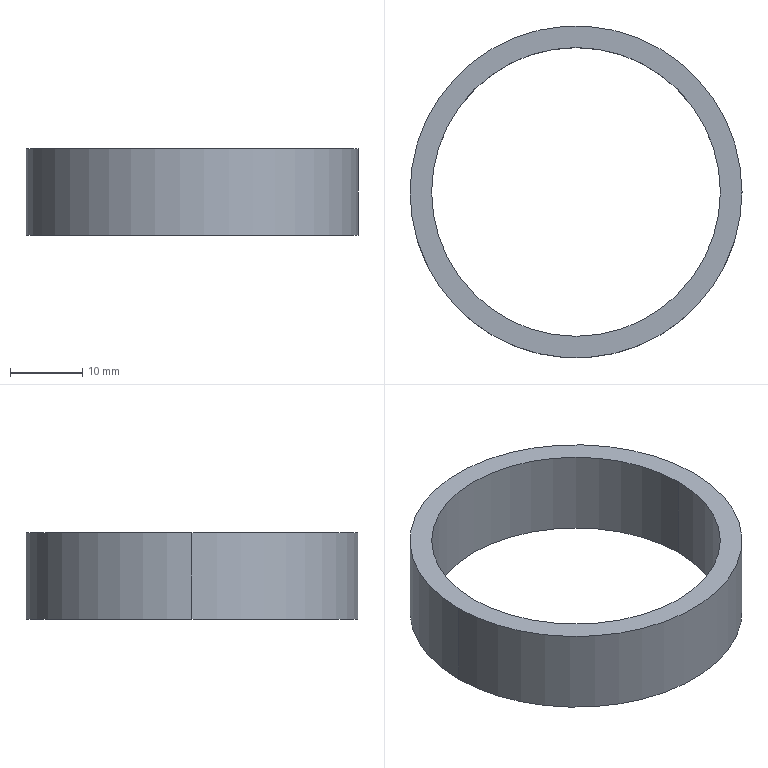Part | SolidWorks | features Extrusion 1 | 1 solid | 6 faces | box 46 x 46 x 12 mm | volume 4863 mm3 | cylinder 4 | plane 2 | commonest cylinder face diameters 40 x2 46 x2
STEP:
#1=CARTESIAN_POINT('',(-20.,0.,12.));
#2=VERTEX_POINT('',#1);
#3=CARTESIAN_POINT('',(20.,0.,12.));
#4=VERTEX_POINT('',#3);
#5=CARTESIAN_POINT('',(0.,0.,12.));
#6=DIRECTION('',(0.,0.,1.));
#7=DIRECTION('',(1.,0.,0.));
#8=AXIS2_PLACEMENT_3D('',#5,#6,#7);
#9=CIRCLE('',#8,20.);
#10=EDGE_CURVE('',#2,#4,#9,.T.);
#11=ORIENTED_EDGE('',*,*,#10,.T.);
#12=CARTESIAN_POINT('',(20.,0.,0.));
#13=VERTEX_POINT('',#12);
#14=CARTESIAN_POINT('',(20.,0.,12.));
#15=DIRECTION('',(0.,0.,-1.));
#16=VECTOR('',#15,1000.);
#17=LINE('',#14,#16);
#18=EDGE_CURVE('',#4,#13,#17,.T.);
#19=ORIENTED_EDGE('',*,*,#18,.T.);
#20=CARTESIAN_POINT('',(-20.,0.,0.));
#21=VERTEX_POINT('',#20);
#22=CARTESIAN_POINT('',(0.,0.,0.));
#23=DIRECTION('',(0.,0.,1.));
#24=DIRECTION('',(1.,0.,0.));
#25=AXIS2_PLACEMENT_3D('',#22,#23,#24);
#26=CIRCLE('',#25,20.);
#27=EDGE_CURVE('',#21,#13,#26,.T.);
#28=ORIENTED_EDGE('',*,*,#27,.F.);
#29=CARTESIAN_POINT('',(-20.,0.,12.));
#30=DIRECTION('',(0.,0.,-1.));
#31=VECTOR('',#30,1000.);
#32=LINE('',#29,#31);
#33=EDGE_CURVE('',#2,#21,#32,.T.);
#34=ORIENTED_EDGE('',*,*,#33,.F.);
#35=EDGE_LOOP('',(#11,#19,#28,#34));
#36=FACE_OUTER_BOUND('',#35,.T.);
#37=CARTESIAN_POINT('',(0.,0.,12.));
#38=DIRECTION('',(0.,0.,-1.));
#39=DIRECTION('',(-1.,0.,0.));
#40=AXIS2_PLACEMENT_3D('',#37,#38,#39);
#41=CYLINDRICAL_SURFACE('',#40,20.);
#42=ADVANCED_FACE('',(#36),#41,.F.);
#43=CARTESIAN_POINT('',(23.,0.,12.));
#44=VERTEX_POINT('',#43);
#45=CARTESIAN_POINT('',(-23.,0.,12.));
#46=VERTEX_POINT('',#45);
#47=CARTESIAN_POINT('',(0.,0.,12.));
#48=DIRECTION('',(0.,0.,1.));
#49=DIRECTION('',(1.,0.,0.));
#50=AXIS2_PLACEMENT_3D('',#47,#48,#49);
#51=CIRCLE('',#50,23.);
#52=EDGE_CURVE('',#44,#46,#51,.T.);
#53=ORIENTED_EDGE('',*,*,#52,.F.);
#54=CARTESIAN_POINT('',(23.,0.,0.));
#55=VERTEX_POINT('',#54);
#56=CARTESIAN_POINT('',(23.,0.,12.));
#57=DIRECTION('',(0.,0.,-1.));
#58=VECTOR('',#57,1000.);
#59=LINE('',#56,#58);
#60=EDGE_CURVE('',#44,#55,#59,.T.);
#61=ORIENTED_EDGE('',*,*,#60,.T.);
#62=CARTESIAN_POINT('',(-23.,0.,0.));
#63=VERTEX_POINT('',#62);
#64=CARTESIAN_POINT('',(0.,0.,0.));
#65=DIRECTION('',(0.,0.,1.));
#66=DIRECTION('',(1.,0.,0.));
#67=AXIS2_PLACEMENT_3D('',#64,#65,#66);
#68=CIRCLE('',#67,23.);
#69=EDGE_CURVE('',#55,#63,#68,.T.);
#70=ORIENTED_EDGE('',*,*,#69,.T.);
#71=CARTESIAN_POINT('',(-23.,0.,12.));
#72=DIRECTION('',(0.,0.,-1.));
#73=VECTOR('',#72,1000.);
#74=LINE('',#71,#73);
#75=EDGE_CURVE('',#46,#63,#74,.T.);
#76=ORIENTED_EDGE('',*,*,#75,.F.);
#77=EDGE_LOOP('',(#53,#61,#70,#76));
#78=FACE_OUTER_BOUND('',#77,.T.);
#79=CARTESIAN_POINT('',(0.,0.,12.));
#80=DIRECTION('',(0.,0.,-1.));
#81=DIRECTION('',(-1.,0.,0.));
#82=AXIS2_PLACEMENT_3D('',#79,#80,#81);
#83=CYLINDRICAL_SURFACE('',#82,23.);
#84=ADVANCED_FACE('',(#78),#83,.T.);
#85=CARTESIAN_POINT('',(0.,0.,12.));
#86=DIRECTION('',(0.,0.,1.));
#87=DIRECTION('',(1.,0.,0.));
#88=AXIS2_PLACEMENT_3D('',#85,#86,#87);
#89=CIRCLE('',#88,23.);
#90=EDGE_CURVE('',#46,#44,#89,.T.);
#91=ORIENTED_EDGE('',*,*,#90,.T.);
#92=ORIENTED_EDGE('',*,*,#52,.T.);
#93=EDGE_LOOP('',(#91,#92));
#94=FACE_OUTER_BOUND('',#93,.T.);
#95=ORIENTED_EDGE('',*,*,#10,.F.);
#96=CARTESIAN_POINT('',(0.,0.,12.));
#97=DIRECTION('',(0.,0.,1.));
#98=DIRECTION('',(1.,0.,0.));
#99=AXIS2_PLACEMENT_3D('',#96,#97,#98);
#100=CIRCLE('',#99,20.);
#101=EDGE_CURVE('',#4,#2,#100,.T.);
#102=ORIENTED_EDGE('',*,*,#101,.F.);
#103=EDGE_LOOP('',(#95,#102));
#104=FACE_BOUND('',#103,.T.);
#105=CARTESIAN_POINT('',(0.,0.,12.));
#106=DIRECTION('',(0.,0.,1.));
#107=DIRECTION('',(1.,0.,0.));
#108=AXIS2_PLACEMENT_3D('',#105,#106,#107);
#109=PLANE('',#108);
#110=ADVANCED_FACE('',(#94,#104),#109,.T.);
#111=CARTESIAN_POINT('',(0.,0.,0.));
#112=DIRECTION('',(0.,0.,1.));
#113=DIRECTION('',(1.,0.,0.));
#114=AXIS2_PLACEMENT_3D('',#111,#112,#113);
#115=CIRCLE('',#114,23.);
#116=EDGE_CURVE('',#63,#55,#115,.T.);
#117=ORIENTED_EDGE('',*,*,#116,.F.);
#118=ORIENTED_EDGE('',*,*,#69,.F.);
#119=EDGE_LOOP('',(#117,#118));
#120=FACE_OUTER_BOUND('',#119,.T.);
#121=ORIENTED_EDGE('',*,*,#27,.T.);
#122=CARTESIAN_POINT('',(0.,0.,0.));
#123=DIRECTION('',(0.,0.,1.));
#124=DIRECTION('',(1.,0.,0.));
#125=AXIS2_PLACEMENT_3D('',#122,#123,#124);
#126=CIRCLE('',#125,20.);
#127=EDGE_CURVE('',#13,#21,#126,.T.);
#128=ORIENTED_EDGE('',*,*,#127,.T.);
#129=EDGE_LOOP('',(#121,#128));
#130=FACE_BOUND('',#129,.T.);
#131=CARTESIAN_POINT('',(0.,0.,0.));
#132=DIRECTION('',(0.,0.,1.));
#133=DIRECTION('',(1.,0.,0.));
#134=AXIS2_PLACEMENT_3D('',#131,#132,#133);
#135=PLANE('',#134);
#136=ADVANCED_FACE('',(#120,#130),#135,.F.);
#137=ORIENTED_EDGE('',*,*,#60,.F.);
#138=ORIENTED_EDGE('',*,*,#90,.F.);
#139=ORIENTED_EDGE('',*,*,#75,.T.);
#140=ORIENTED_EDGE('',*,*,#116,.T.);
#141=EDGE_LOOP('',(#137,#138,#139,#140));
#142=FACE_OUTER_BOUND('',#141,.T.);
#143=CARTESIAN_POINT('',(0.,0.,12.));
#144=DIRECTION('',(0.,0.,-1.));
#145=DIRECTION('',(-1.,0.,0.));
#146=AXIS2_PLACEMENT_3D('',#143,#144,#145);
#147=CYLINDRICAL_SURFACE('',#146,23.);
#148=ADVANCED_FACE('',(#142),#147,.T.);
#149=ORIENTED_EDGE('',*,*,#18,.F.);
#150=ORIENTED_EDGE('',*,*,#101,.T.);
#151=ORIENTED_EDGE('',*,*,#33,.T.);
#152=ORIENTED_EDGE('',*,*,#127,.F.);
#153=EDGE_LOOP('',(#149,#150,#151,#152));
#154=FACE_OUTER_BOUND('',#153,.T.);
#155=CARTESIAN_POINT('',(0.,0.,12.));
#156=DIRECTION('',(0.,0.,-1.));
#157=DIRECTION('',(-1.,0.,0.));
#158=AXIS2_PLACEMENT_3D('',#155,#156,#157);
#159=CYLINDRICAL_SURFACE('',#158,20.);
#160=ADVANCED_FACE('',(#154),#159,.F.);
#161=CLOSED_SHELL('',(#42,#84,#110,#136,#148,#160));
#162=MANIFOLD_SOLID_BREP('',#161);
#163=CARTESIAN_POINT('',(0.,0.,0.));
#164=DIRECTION('',(0.,0.,1.));
#165=DIRECTION('',(1.,0.,0.));
#166=AXIS2_PLACEMENT_3D('',#163,#164,#165);
#167=(LENGTH_UNIT()NAMED_UNIT(*)SI_UNIT(.MILLI.,.METRE.));
#168=UNCERTAINTY_MEASURE_WITH_UNIT(LENGTH_MEASURE(0.00001),#167,'','');
#169=(NAMED_UNIT(*)PLANE_ANGLE_UNIT()SI_UNIT($,.RADIAN.));
#170=(NAMED_UNIT(*)SI_UNIT($,.STERADIAN.)SOLID_ANGLE_UNIT());
#171=(GEOMETRIC_REPRESENTATION_CONTEXT(3)GLOBAL_UNCERTAINTY_ASSIGNED_CONTEXT((#168))GLOBAL_UNIT_ASSIGNED_CONTEXT((#167,#169,#170))REPRESENTATION_CONTEXT('',''));
#172=ADVANCED_BREP_SHAPE_REPRESENTATION('',(#162,#166),#171);